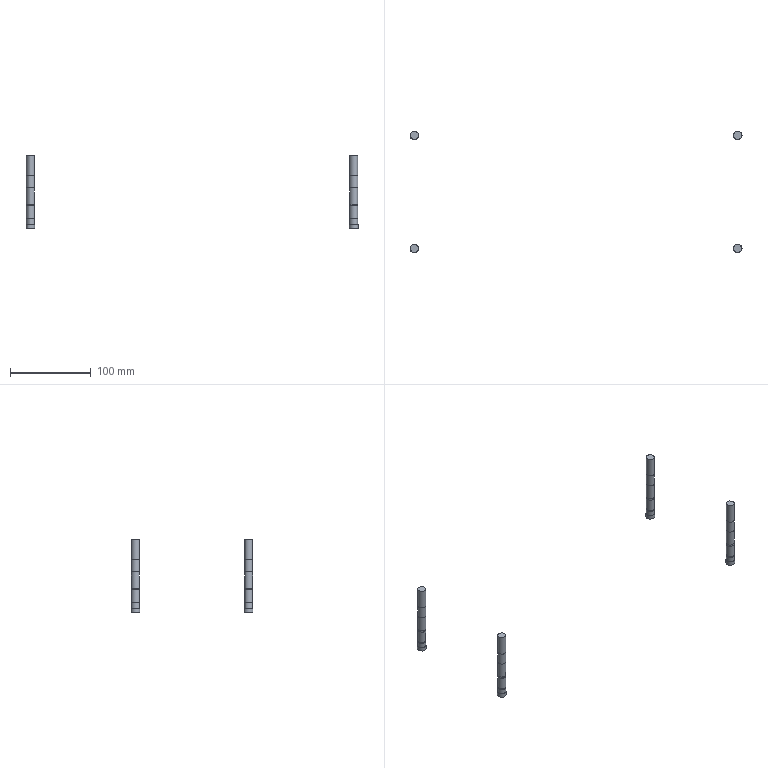Part | NX | features BREP 2 | 8 solids | 56 faces | box 410.8 x 150.8 x 90 mm | volume 34728 mm3 | plane 28 | cylinder 20 | torus 4 | cone 4 | commonest cylinder face diameters 10 x8 10.008 x4 10.1 x4 10.8 x4